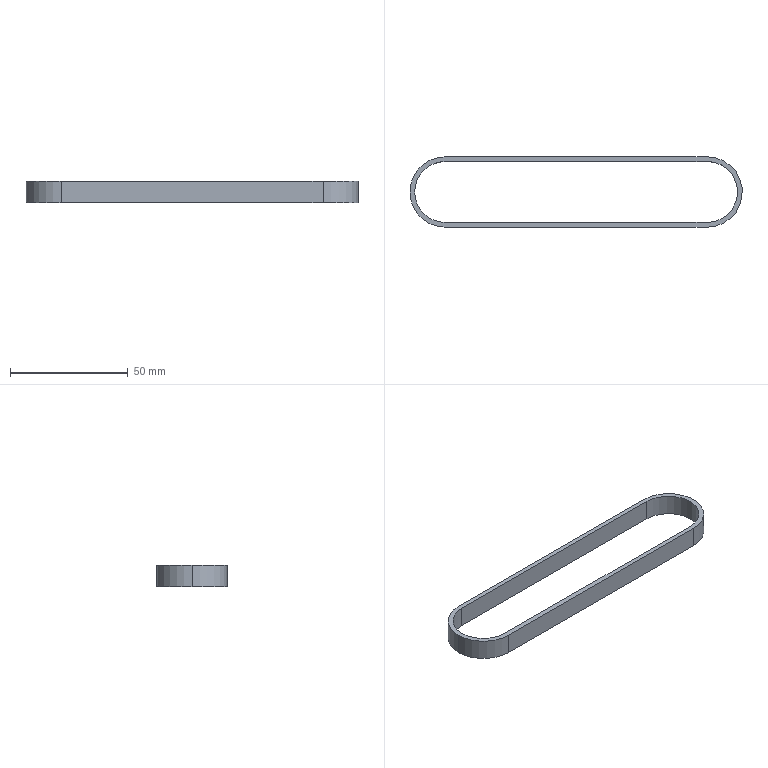Part | NX | features BREP 1 | 1 solid | 12 faces | box 140.87 x 29.87 x 9 mm | volume 5572 mm3 | cylinder 6 | plane 6 | commonest cylinder face diameters 25.87 x3 29.87 x3
STEP:
#1=CARTESIAN_POINT('',(0.,12.935,9.));
#2=VERTEX_POINT('',#1);
#3=CARTESIAN_POINT('',(-12.935,0.,9.));
#4=VERTEX_POINT('',#3);
#5=CARTESIAN_POINT('',(0.,0.,9.));
#6=DIRECTION('',(0.,0.,1.));
#7=DIRECTION('',(1.,0.,0.));
#8=AXIS2_PLACEMENT_3D('',#5,#6,#7);
#9=CIRCLE('',#8,12.935);
#10=EDGE_CURVE('',#2,#4,#9,.T.);
#11=ORIENTED_EDGE('',*,*,#10,.T.);
#12=CARTESIAN_POINT('',(-12.935,0.,0.));
#13=VERTEX_POINT('',#12);
#14=CARTESIAN_POINT('',(-12.935,0.,9.));
#15=DIRECTION('',(0.,0.,-1.));
#16=VECTOR('',#15,1000.);
#17=LINE('',#14,#16);
#18=EDGE_CURVE('',#4,#13,#17,.T.);
#19=ORIENTED_EDGE('',*,*,#18,.T.);
#20=CARTESIAN_POINT('',(0.,12.935,0.));
#21=VERTEX_POINT('',#20);
#22=CARTESIAN_POINT('',(0.,0.,0.));
#23=DIRECTION('',(0.,0.,1.));
#24=DIRECTION('',(1.,0.,0.));
#25=AXIS2_PLACEMENT_3D('',#22,#23,#24);
#26=CIRCLE('',#25,12.935);
#27=EDGE_CURVE('',#21,#13,#26,.T.);
#28=ORIENTED_EDGE('',*,*,#27,.F.);
#29=CARTESIAN_POINT('',(0.,12.935,9.));
#30=DIRECTION('',(0.,0.,-1.));
#31=VECTOR('',#30,1000.);
#32=LINE('',#29,#31);
#33=EDGE_CURVE('',#2,#21,#32,.T.);
#34=ORIENTED_EDGE('',*,*,#33,.F.);
#35=EDGE_LOOP('',(#11,#19,#28,#34));
#36=FACE_BOUND('',#35,.T.);
#37=CARTESIAN_POINT('',(0.,0.,9.));
#38=DIRECTION('',(0.,0.,-1.));
#39=DIRECTION('',(-1.,0.,0.));
#40=AXIS2_PLACEMENT_3D('',#37,#38,#39);
#41=CYLINDRICAL_SURFACE('',#40,12.935);
#42=ADVANCED_FACE('',(#36),#41,.F.);
#43=CARTESIAN_POINT('',(-14.935,0.,9.));
#44=VERTEX_POINT('',#43);
#45=CARTESIAN_POINT('',(0.,-14.935,9.));
#46=VERTEX_POINT('',#45);
#47=CARTESIAN_POINT('',(0.,0.,9.));
#48=DIRECTION('',(0.,0.,1.));
#49=DIRECTION('',(1.,0.,0.));
#50=AXIS2_PLACEMENT_3D('',#47,#48,#49);
#51=CIRCLE('',#50,14.935);
#52=EDGE_CURVE('',#44,#46,#51,.T.);
#53=ORIENTED_EDGE('',*,*,#52,.F.);
#54=CARTESIAN_POINT('',(-14.935,0.,0.));
#55=VERTEX_POINT('',#54);
#56=CARTESIAN_POINT('',(-14.935,0.,9.));
#57=DIRECTION('',(0.,0.,-1.));
#58=VECTOR('',#57,1000.);
#59=LINE('',#56,#58);
#60=EDGE_CURVE('',#44,#55,#59,.T.);
#61=ORIENTED_EDGE('',*,*,#60,.T.);
#62=CARTESIAN_POINT('',(0.,-14.935,0.));
#63=VERTEX_POINT('',#62);
#64=CARTESIAN_POINT('',(0.,0.,0.));
#65=DIRECTION('',(0.,0.,1.));
#66=DIRECTION('',(1.,0.,0.));
#67=AXIS2_PLACEMENT_3D('',#64,#65,#66);
#68=CIRCLE('',#67,14.935);
#69=EDGE_CURVE('',#55,#63,#68,.T.);
#70=ORIENTED_EDGE('',*,*,#69,.T.);
#71=CARTESIAN_POINT('',(0.,-14.935,9.));
#72=DIRECTION('',(0.,0.,-1.));
#73=VECTOR('',#72,1000.);
#74=LINE('',#71,#73);
#75=EDGE_CURVE('',#46,#63,#74,.T.);
#76=ORIENTED_EDGE('',*,*,#75,.F.);
#77=EDGE_LOOP('',(#53,#61,#70,#76));
#78=FACE_BOUND('',#77,.T.);
#79=CARTESIAN_POINT('',(0.,0.,9.));
#80=DIRECTION('',(0.,0.,-1.));
#81=DIRECTION('',(-1.,0.,0.));
#82=AXIS2_PLACEMENT_3D('',#79,#80,#81);
#83=CYLINDRICAL_SURFACE('',#82,14.935);
#84=ADVANCED_FACE('',(#78),#83,.T.);
#85=CARTESIAN_POINT('',(0.,14.935,9.));
#86=VERTEX_POINT('',#85);
#87=CARTESIAN_POINT('',(0.,0.,9.));
#88=DIRECTION('',(0.,0.,1.));
#89=DIRECTION('',(1.,0.,0.));
#90=AXIS2_PLACEMENT_3D('',#87,#88,#89);
#91=CIRCLE('',#90,14.935);
#92=EDGE_CURVE('',#86,#44,#91,.T.);
#93=ORIENTED_EDGE('',*,*,#92,.T.);
#94=ORIENTED_EDGE('',*,*,#52,.T.);
#95=CARTESIAN_POINT('',(111.,-14.935,9.));
#96=VERTEX_POINT('',#95);
#97=CARTESIAN_POINT('',(0.,-14.935,9.));
#98=DIRECTION('',(1.,0.,0.));
#99=VECTOR('',#98,1000.);
#100=LINE('',#97,#99);
#101=EDGE_CURVE('',#46,#96,#100,.T.);
#102=ORIENTED_EDGE('',*,*,#101,.T.);
#103=CARTESIAN_POINT('',(111.,14.935,9.));
#104=VERTEX_POINT('',#103);
#105=CARTESIAN_POINT('',(111.,0.,9.));
#106=DIRECTION('',(0.,0.,1.));
#107=DIRECTION('',(1.,0.,0.));
#108=AXIS2_PLACEMENT_3D('',#105,#106,#107);
#109=CIRCLE('',#108,14.935);
#110=EDGE_CURVE('',#96,#104,#109,.T.);
#111=ORIENTED_EDGE('',*,*,#110,.T.);
#112=CARTESIAN_POINT('',(0.,14.935,9.));
#113=DIRECTION('',(-1.,0.,0.));
#114=VECTOR('',#113,1000.);
#115=LINE('',#112,#114);
#116=EDGE_CURVE('',#104,#86,#115,.T.);
#117=ORIENTED_EDGE('',*,*,#116,.T.);
#118=EDGE_LOOP('',(#93,#94,#102,#111,#117));
#119=FACE_BOUND('',#118,.T.);
#120=CARTESIAN_POINT('',(0.,-12.935,9.));
#121=VERTEX_POINT('',#120);
#122=CARTESIAN_POINT('',(111.,-12.935,9.));
#123=VERTEX_POINT('',#122);
#124=CARTESIAN_POINT('',(0.,-12.935,9.));
#125=DIRECTION('',(1.,0.,0.));
#126=VECTOR('',#125,1000.);
#127=LINE('',#124,#126);
#128=EDGE_CURVE('',#121,#123,#127,.T.);
#129=ORIENTED_EDGE('',*,*,#128,.F.);
#130=CARTESIAN_POINT('',(0.,0.,9.));
#131=DIRECTION('',(0.,0.,1.));
#132=DIRECTION('',(1.,0.,0.));
#133=AXIS2_PLACEMENT_3D('',#130,#131,#132);
#134=CIRCLE('',#133,12.935);
#135=EDGE_CURVE('',#4,#121,#134,.T.);
#136=ORIENTED_EDGE('',*,*,#135,.F.);
#137=ORIENTED_EDGE('',*,*,#10,.F.);
#138=CARTESIAN_POINT('',(111.,12.935,9.));
#139=VERTEX_POINT('',#138);
#140=CARTESIAN_POINT('',(0.,12.935,9.));
#141=DIRECTION('',(-1.,0.,0.));
#142=VECTOR('',#141,1000.);
#143=LINE('',#140,#142);
#144=EDGE_CURVE('',#139,#2,#143,.T.);
#145=ORIENTED_EDGE('',*,*,#144,.F.);
#146=CARTESIAN_POINT('',(111.,0.,9.));
#147=DIRECTION('',(0.,0.,1.));
#148=DIRECTION('',(1.,0.,0.));
#149=AXIS2_PLACEMENT_3D('',#146,#147,#148);
#150=CIRCLE('',#149,12.935);
#151=EDGE_CURVE('',#123,#139,#150,.T.);
#152=ORIENTED_EDGE('',*,*,#151,.F.);
#153=EDGE_LOOP('',(#129,#136,#137,#145,#152));
#154=FACE_BOUND('',#153,.T.);
#155=CARTESIAN_POINT('',(0.,0.,9.));
#156=DIRECTION('',(0.,0.,1.));
#157=DIRECTION('',(1.,0.,0.));
#158=AXIS2_PLACEMENT_3D('',#155,#156,#157);
#159=PLANE('',#158);
#160=ADVANCED_FACE('',(#119,#154),#159,.T.);
#161=CARTESIAN_POINT('',(0.,14.935,0.));
#162=VERTEX_POINT('',#161);
#163=CARTESIAN_POINT('',(0.,0.,0.));
#164=DIRECTION('',(0.,0.,1.));
#165=DIRECTION('',(1.,0.,0.));
#166=AXIS2_PLACEMENT_3D('',#163,#164,#165);
#167=CIRCLE('',#166,14.935);
#168=EDGE_CURVE('',#162,#55,#167,.T.);
#169=ORIENTED_EDGE('',*,*,#168,.F.);
#170=CARTESIAN_POINT('',(111.,14.935,0.));
#171=VERTEX_POINT('',#170);
#172=CARTESIAN_POINT('',(0.,14.935,0.));
#173=DIRECTION('',(-1.,0.,0.));
#174=VECTOR('',#173,1000.);
#175=LINE('',#172,#174);
#176=EDGE_CURVE('',#171,#162,#175,.T.);
#177=ORIENTED_EDGE('',*,*,#176,.F.);
#178=CARTESIAN_POINT('',(111.,-14.935,0.));
#179=VERTEX_POINT('',#178);
#180=CARTESIAN_POINT('',(111.,0.,0.));
#181=DIRECTION('',(0.,0.,1.));
#182=DIRECTION('',(1.,0.,0.));
#183=AXIS2_PLACEMENT_3D('',#180,#181,#182);
#184=CIRCLE('',#183,14.935);
#185=EDGE_CURVE('',#179,#171,#184,.T.);
#186=ORIENTED_EDGE('',*,*,#185,.F.);
#187=CARTESIAN_POINT('',(0.,-14.935,0.));
#188=DIRECTION('',(1.,0.,0.));
#189=VECTOR('',#188,1000.);
#190=LINE('',#187,#189);
#191=EDGE_CURVE('',#63,#179,#190,.T.);
#192=ORIENTED_EDGE('',*,*,#191,.F.);
#193=ORIENTED_EDGE('',*,*,#69,.F.);
#194=EDGE_LOOP('',(#169,#177,#186,#192,#193));
#195=FACE_BOUND('',#194,.T.);
#196=ORIENTED_EDGE('',*,*,#27,.T.);
#197=CARTESIAN_POINT('',(0.,-12.935,0.));
#198=VERTEX_POINT('',#197);
#199=CARTESIAN_POINT('',(0.,0.,0.));
#200=DIRECTION('',(0.,0.,1.));
#201=DIRECTION('',(1.,0.,0.));
#202=AXIS2_PLACEMENT_3D('',#199,#200,#201);
#203=CIRCLE('',#202,12.935);
#204=EDGE_CURVE('',#13,#198,#203,.T.);
#205=ORIENTED_EDGE('',*,*,#204,.T.);
#206=CARTESIAN_POINT('',(111.,-12.935,0.));
#207=VERTEX_POINT('',#206);
#208=CARTESIAN_POINT('',(0.,-12.935,0.));
#209=DIRECTION('',(1.,0.,0.));
#210=VECTOR('',#209,1000.);
#211=LINE('',#208,#210);
#212=EDGE_CURVE('',#198,#207,#211,.T.);
#213=ORIENTED_EDGE('',*,*,#212,.T.);
#214=CARTESIAN_POINT('',(111.,12.935,0.));
#215=VERTEX_POINT('',#214);
#216=CARTESIAN_POINT('',(111.,0.,0.));
#217=DIRECTION('',(0.,0.,1.));
#218=DIRECTION('',(1.,0.,0.));
#219=AXIS2_PLACEMENT_3D('',#216,#217,#218);
#220=CIRCLE('',#219,12.935);
#221=EDGE_CURVE('',#207,#215,#220,.T.);
#222=ORIENTED_EDGE('',*,*,#221,.T.);
#223=CARTESIAN_POINT('',(0.,12.935,0.));
#224=DIRECTION('',(-1.,0.,0.));
#225=VECTOR('',#224,1000.);
#226=LINE('',#223,#225);
#227=EDGE_CURVE('',#215,#21,#226,.T.);
#228=ORIENTED_EDGE('',*,*,#227,.T.);
#229=EDGE_LOOP('',(#196,#205,#213,#222,#228));
#230=FACE_BOUND('',#229,.T.);
#231=CARTESIAN_POINT('',(0.,0.,0.));
#232=DIRECTION('',(0.,0.,1.));
#233=DIRECTION('',(1.,0.,0.));
#234=AXIS2_PLACEMENT_3D('',#231,#232,#233);
#235=PLANE('',#234);
#236=ADVANCED_FACE('',(#195,#230),#235,.F.);
#237=ORIENTED_EDGE('',*,*,#60,.F.);
#238=ORIENTED_EDGE('',*,*,#92,.F.);
#239=CARTESIAN_POINT('',(0.,14.935,9.));
#240=DIRECTION('',(0.,0.,-1.));
#241=VECTOR('',#240,1000.);
#242=LINE('',#239,#241);
#243=EDGE_CURVE('',#86,#162,#242,.T.);
#244=ORIENTED_EDGE('',*,*,#243,.T.);
#245=ORIENTED_EDGE('',*,*,#168,.T.);
#246=EDGE_LOOP('',(#237,#238,#244,#245));
#247=FACE_BOUND('',#246,.T.);
#248=CARTESIAN_POINT('',(0.,0.,9.));
#249=DIRECTION('',(0.,0.,-1.));
#250=DIRECTION('',(-1.,0.,0.));
#251=AXIS2_PLACEMENT_3D('',#248,#249,#250);
#252=CYLINDRICAL_SURFACE('',#251,14.935);
#253=ADVANCED_FACE('',(#247),#252,.T.);
#254=ORIENTED_EDGE('',*,*,#191,.T.);
#255=CARTESIAN_POINT('',(111.,-14.935,9.));
#256=DIRECTION('',(0.,0.,-1.));
#257=VECTOR('',#256,1000.);
#258=LINE('',#255,#257);
#259=EDGE_CURVE('',#96,#179,#258,.T.);
#260=ORIENTED_EDGE('',*,*,#259,.F.);
#261=ORIENTED_EDGE('',*,*,#101,.F.);
#262=ORIENTED_EDGE('',*,*,#75,.T.);
#263=EDGE_LOOP('',(#254,#260,#261,#262));
#264=FACE_BOUND('',#263,.T.);
#265=CARTESIAN_POINT('',(0.,-14.935,9.));
#266=DIRECTION('',(0.,1.,0.));
#267=DIRECTION('',(1.,0.,0.));
#268=AXIS2_PLACEMENT_3D('',#265,#266,#267);
#269=PLANE('',#268);
#270=ADVANCED_FACE('',(#264),#269,.F.);
#271=ORIENTED_EDGE('',*,*,#185,.T.);
#272=CARTESIAN_POINT('',(111.,14.935,9.));
#273=DIRECTION('',(0.,0.,-1.));
#274=VECTOR('',#273,1000.);
#275=LINE('',#272,#274);
#276=EDGE_CURVE('',#104,#171,#275,.T.);
#277=ORIENTED_EDGE('',*,*,#276,.F.);
#278=ORIENTED_EDGE('',*,*,#110,.F.);
#279=ORIENTED_EDGE('',*,*,#259,.T.);
#280=EDGE_LOOP('',(#271,#277,#278,#279));
#281=FACE_BOUND('',#280,.T.);
#282=CARTESIAN_POINT('',(111.,0.,9.));
#283=DIRECTION('',(0.,0.,-1.));
#284=DIRECTION('',(-1.,0.,0.));
#285=AXIS2_PLACEMENT_3D('',#282,#283,#284);
#286=CYLINDRICAL_SURFACE('',#285,14.935);
#287=ADVANCED_FACE('',(#281),#286,.T.);
#288=ORIENTED_EDGE('',*,*,#176,.T.);
#289=ORIENTED_EDGE('',*,*,#243,.F.);
#290=ORIENTED_EDGE('',*,*,#116,.F.);
#291=ORIENTED_EDGE('',*,*,#276,.T.);
#292=EDGE_LOOP('',(#288,#289,#290,#291));
#293=FACE_BOUND('',#292,.T.);
#294=CARTESIAN_POINT('',(0.,14.935,9.));
#295=DIRECTION('',(0.,-1.,0.));
#296=DIRECTION('',(-1.,0.,0.));
#297=AXIS2_PLACEMENT_3D('',#294,#295,#296);
#298=PLANE('',#297);
#299=ADVANCED_FACE('',(#293),#298,.F.);
#300=ORIENTED_EDGE('',*,*,#18,.F.);
#301=ORIENTED_EDGE('',*,*,#135,.T.);
#302=CARTESIAN_POINT('',(0.,-12.935,9.));
#303=DIRECTION('',(0.,0.,-1.));
#304=VECTOR('',#303,1000.);
#305=LINE('',#302,#304);
#306=EDGE_CURVE('',#121,#198,#305,.T.);
#307=ORIENTED_EDGE('',*,*,#306,.T.);
#308=ORIENTED_EDGE('',*,*,#204,.F.);
#309=EDGE_LOOP('',(#300,#301,#307,#308));
#310=FACE_BOUND('',#309,.T.);
#311=CARTESIAN_POINT('',(0.,0.,9.));
#312=DIRECTION('',(0.,0.,-1.));
#313=DIRECTION('',(-1.,0.,0.));
#314=AXIS2_PLACEMENT_3D('',#311,#312,#313);
#315=CYLINDRICAL_SURFACE('',#314,12.935);
#316=ADVANCED_FACE('',(#310),#315,.F.);
#317=ORIENTED_EDGE('',*,*,#212,.F.);
#318=ORIENTED_EDGE('',*,*,#306,.F.);
#319=ORIENTED_EDGE('',*,*,#128,.T.);
#320=CARTESIAN_POINT('',(111.,-12.935,9.));
#321=DIRECTION('',(0.,0.,-1.));
#322=VECTOR('',#321,1000.);
#323=LINE('',#320,#322);
#324=EDGE_CURVE('',#123,#207,#323,.T.);
#325=ORIENTED_EDGE('',*,*,#324,.T.);
#326=EDGE_LOOP('',(#317,#318,#319,#325));
#327=FACE_BOUND('',#326,.T.);
#328=CARTESIAN_POINT('',(0.,-12.935,9.));
#329=DIRECTION('',(0.,1.,0.));
#330=DIRECTION('',(1.,0.,0.));
#331=AXIS2_PLACEMENT_3D('',#328,#329,#330);
#332=PLANE('',#331);
#333=ADVANCED_FACE('',(#327),#332,.T.);
#334=ORIENTED_EDGE('',*,*,#221,.F.);
#335=ORIENTED_EDGE('',*,*,#324,.F.);
#336=ORIENTED_EDGE('',*,*,#151,.T.);
#337=CARTESIAN_POINT('',(111.,12.935,9.));
#338=DIRECTION('',(0.,0.,-1.));
#339=VECTOR('',#338,1000.);
#340=LINE('',#337,#339);
#341=EDGE_CURVE('',#139,#215,#340,.T.);
#342=ORIENTED_EDGE('',*,*,#341,.T.);
#343=EDGE_LOOP('',(#334,#335,#336,#342));
#344=FACE_BOUND('',#343,.T.);
#345=CARTESIAN_POINT('',(111.,0.,9.));
#346=DIRECTION('',(0.,0.,-1.));
#347=DIRECTION('',(-1.,0.,0.));
#348=AXIS2_PLACEMENT_3D('',#345,#346,#347);
#349=CYLINDRICAL_SURFACE('',#348,12.935);
#350=ADVANCED_FACE('',(#344),#349,.F.);
#351=ORIENTED_EDGE('',*,*,#227,.F.);
#352=ORIENTED_EDGE('',*,*,#341,.F.);
#353=ORIENTED_EDGE('',*,*,#144,.T.);
#354=ORIENTED_EDGE('',*,*,#33,.T.);
#355=EDGE_LOOP('',(#351,#352,#353,#354));
#356=FACE_BOUND('',#355,.T.);
#357=CARTESIAN_POINT('',(0.,12.935,9.));
#358=DIRECTION('',(0.,-1.,0.));
#359=DIRECTION('',(0.,0.,-1.));
#360=AXIS2_PLACEMENT_3D('',#357,#358,#359);
#361=PLANE('',#360);
#362=ADVANCED_FACE('',(#356),#361,.T.);
#363=CLOSED_SHELL('',(#42,#84,#160,#236,#253,#270,#287,#299,#316,#333,#350,#362));
#364=MANIFOLD_SOLID_BREP('',#363);
#365=(LENGTH_UNIT()NAMED_UNIT(*)SI_UNIT(.MILLI.,.METRE.));
#366=UNCERTAINTY_MEASURE_WITH_UNIT(LENGTH_MEASURE(0.00001),#365,'','');
#367=(NAMED_UNIT(*)PLANE_ANGLE_UNIT()SI_UNIT($,.RADIAN.));
#368=(NAMED_UNIT(*)SI_UNIT($,.STERADIAN.)SOLID_ANGLE_UNIT());
#369=(GEOMETRIC_REPRESENTATION_CONTEXT(3)GLOBAL_UNCERTAINTY_ASSIGNED_CONTEXT((#366))GLOBAL_UNIT_ASSIGNED_CONTEXT((#365,#367,#368))REPRESENTATION_CONTEXT('',''));
#370=ADVANCED_BREP_SHAPE_REPRESENTATION('',(#364),#369);